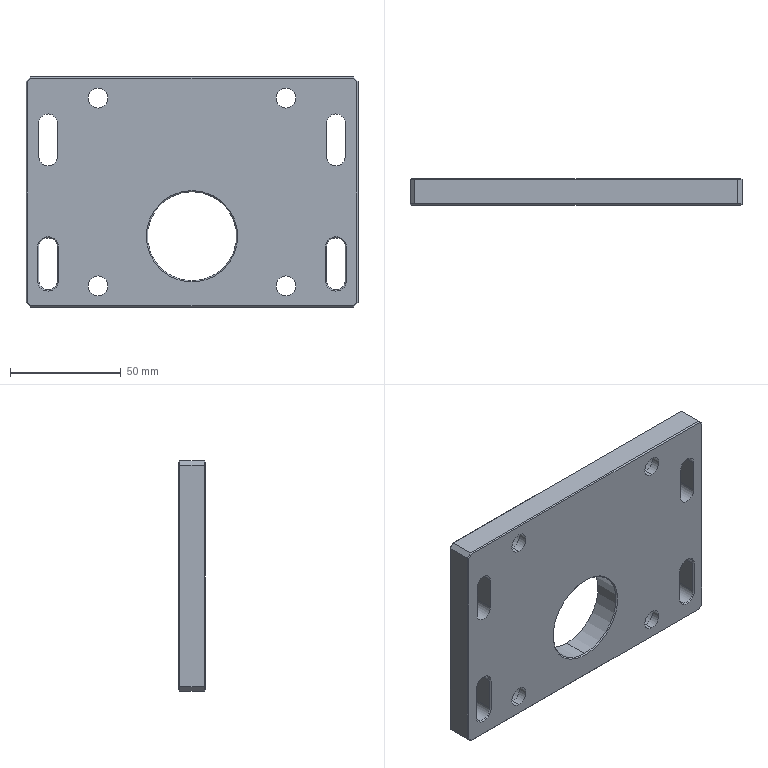Part | STEP file | 180W motor mounting plate_Default | 1 solid | 80 faces | box 150 x 12 x 104 mm | volume 156125 mm3 | plane 42 | cylinder 30 | cone 8 | commonest cylinder face diameters 8.5 x12 9 x8 15 x8 40.3 x2